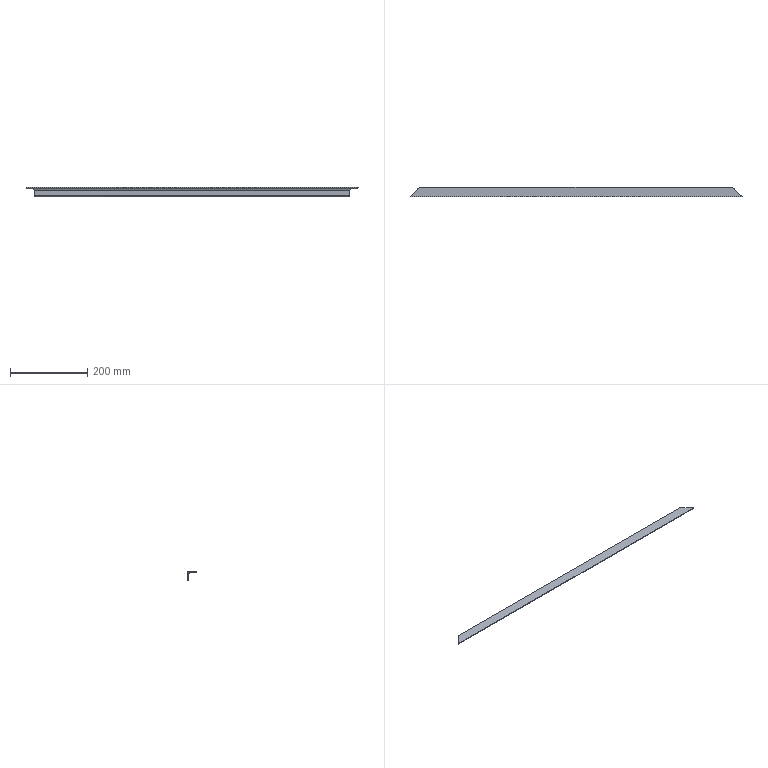Part | STEP file | Guide wheel mechanism revised.sldasm-Part-17 | 1 solid | 9 faces | box 860 x 25 x 25 mm | volume 148281 mm3 | plane 6 | cylinder 3 | commonest cylinder face diameters 8 x2 7 x1
STEP:
#1=CARTESIAN_POINT('',(-430.,795.,-505.));
#2=VERTEX_POINT('',#1);
#3=CARTESIAN_POINT('',(-405.,820.,-505.));
#4=VERTEX_POINT('',#3);
#5=CARTESIAN_POINT('',(-12.5,1212.5,-505.));
#6=DIRECTION('',(0.7071,0.7071,0.));
#7=VECTOR('',#6,1000.);
#8=LINE('',#5,#7);
#9=EDGE_CURVE('',#2,#4,#8,.T.);
#10=ORIENTED_EDGE('',*,*,#9,.F.);
#11=CARTESIAN_POINT('',(430.,795.,-505.));
#12=VERTEX_POINT('',#11);
#13=CARTESIAN_POINT('',(405.,795.,-505.));
#14=DIRECTION('',(-1.,0.,0.));
#15=VECTOR('',#14,1000.);
#16=LINE('',#13,#15);
#17=EDGE_CURVE('',#12,#2,#16,.T.);
#18=ORIENTED_EDGE('',*,*,#17,.F.);
#19=CARTESIAN_POINT('',(405.,820.,-505.));
#20=VERTEX_POINT('',#19);
#21=CARTESIAN_POINT('',(417.5,807.5,-505.));
#22=DIRECTION('',(0.7071,-0.7071,0.));
#23=VECTOR('',#22,1000.);
#24=LINE('',#21,#23);
#25=EDGE_CURVE('',#20,#12,#24,.T.);
#26=ORIENTED_EDGE('',*,*,#25,.F.);
#27=CARTESIAN_POINT('',(405.,820.,-505.));
#28=DIRECTION('',(-1.,0.,0.));
#29=VECTOR('',#28,1000.);
#30=LINE('',#27,#29);
#31=EDGE_CURVE('',#20,#4,#30,.T.);
#32=ORIENTED_EDGE('',*,*,#31,.T.);
#33=EDGE_LOOP('',(#10,#18,#26,#32));
#34=FACE_OUTER_BOUND('',#33,.T.);
#35=CARTESIAN_POINT('',(405.,795.,-505.));
#36=DIRECTION('',(0.,0.,-1.));
#37=DIRECTION('',(-1.,0.,0.));
#38=AXIS2_PLACEMENT_3D('',#35,#36,#37);
#39=PLANE('',#38);
#40=ADVANCED_FACE('',(#34),#39,.F.);
#41=CARTESIAN_POINT('',(-426.,799.,-509.));
#42=VERTEX_POINT('',#41);
#43=CARTESIAN_POINT('',(-426.,799.,-509.));
#44=CARTESIAN_POINT('',(-428.343,796.657,-509.));
#45=CARTESIAN_POINT('',(-430.,795.,-507.343));
#46=CARTESIAN_POINT('',(-430.,795.,-505.));
#47=(BOUNDED_CURVE()B_SPLINE_CURVE(3,(#43,#44,#45,#46),.UNSPECIFIED.,.F.,.F.)B_SPLINE_CURVE_WITH_KNOTS((4,4),(4.712,6.283),.UNSPECIFIED.)CURVE()GEOMETRIC_REPRESENTATION_ITEM()RATIONAL_B_SPLINE_CURVE((1.,0.8047,0.8047,1.))REPRESENTATION_ITEM(''));
#48=EDGE_CURVE('',#42,#2,#47,.T.);
#49=ORIENTED_EDGE('',*,*,#48,.F.);
#50=CARTESIAN_POINT('',(426.,799.,-509.));
#51=VERTEX_POINT('',#50);
#52=CARTESIAN_POINT('',(405.,799.,-509.));
#53=DIRECTION('',(-1.,0.,0.));
#54=VECTOR('',#53,1000.);
#55=LINE('',#52,#54);
#56=EDGE_CURVE('',#51,#42,#55,.T.);
#57=ORIENTED_EDGE('',*,*,#56,.F.);
#58=CARTESIAN_POINT('',(430.,795.,-505.));
#59=CARTESIAN_POINT('',(430.,795.,-507.343));
#60=CARTESIAN_POINT('',(428.343,796.657,-509.));
#61=CARTESIAN_POINT('',(426.,799.,-509.));
#62=(BOUNDED_CURVE()B_SPLINE_CURVE(3,(#58,#59,#60,#61),.UNSPECIFIED.,.F.,.F.)B_SPLINE_CURVE_WITH_KNOTS((4,4),(3.142,4.712),.UNSPECIFIED.)CURVE()GEOMETRIC_REPRESENTATION_ITEM()RATIONAL_B_SPLINE_CURVE((1.,0.8047,0.8047,1.))REPRESENTATION_ITEM(''));
#63=EDGE_CURVE('',#12,#51,#62,.T.);
#64=ORIENTED_EDGE('',*,*,#63,.F.);
#65=ORIENTED_EDGE('',*,*,#17,.T.);
#66=EDGE_LOOP('',(#49,#57,#64,#65));
#67=FACE_OUTER_BOUND('',#66,.T.);
#68=CARTESIAN_POINT('',(405.,799.,-505.));
#69=DIRECTION('',(-1.,0.,0.));
#70=DIRECTION('',(0.,0.,1.));
#71=AXIS2_PLACEMENT_3D('',#68,#69,#70);
#72=CYLINDRICAL_SURFACE('',#71,4.);
#73=ADVANCED_FACE('',(#67),#72,.T.);
#74=CARTESIAN_POINT('',(-412.5,812.5,-509.));
#75=VERTEX_POINT('',#74);
#76=CARTESIAN_POINT('',(-3.75,1221.25,-509.));
#77=DIRECTION('',(-0.7071,-0.7071,0.));
#78=VECTOR('',#77,1000.);
#79=LINE('',#76,#78);
#80=EDGE_CURVE('',#75,#42,#79,.T.);
#81=ORIENTED_EDGE('',*,*,#80,.F.);
#82=CARTESIAN_POINT('',(412.5,812.5,-509.));
#83=VERTEX_POINT('',#82);
#84=CARTESIAN_POINT('',(405.,812.5,-509.));
#85=DIRECTION('',(-1.,0.,0.));
#86=VECTOR('',#85,1000.);
#87=LINE('',#84,#86);
#88=EDGE_CURVE('',#83,#75,#87,.T.);
#89=ORIENTED_EDGE('',*,*,#88,.F.);
#90=CARTESIAN_POINT('',(408.75,816.25,-509.));
#91=DIRECTION('',(-0.7071,0.7071,0.));
#92=VECTOR('',#91,1000.);
#93=LINE('',#90,#92);
#94=EDGE_CURVE('',#51,#83,#93,.T.);
#95=ORIENTED_EDGE('',*,*,#94,.F.);
#96=ORIENTED_EDGE('',*,*,#56,.T.);
#97=EDGE_LOOP('',(#81,#89,#95,#96));
#98=FACE_OUTER_BOUND('',#97,.T.);
#99=CARTESIAN_POINT('',(405.,812.5,-509.));
#100=DIRECTION('',(0.,0.,1.));
#101=DIRECTION('',(1.,0.,0.));
#102=AXIS2_PLACEMENT_3D('',#99,#100,#101);
#103=PLANE('',#102);
#104=ADVANCED_FACE('',(#98),#103,.F.);
#105=CARTESIAN_POINT('',(-409.,816.,-512.5));
#106=VERTEX_POINT('',#105);
#107=CARTESIAN_POINT('',(-409.,816.,-512.5));
#108=CARTESIAN_POINT('',(-409.,816.,-510.45));
#109=CARTESIAN_POINT('',(-410.45,814.55,-509.));
#110=CARTESIAN_POINT('',(-412.5,812.5,-509.));
#111=(BOUNDED_CURVE()B_SPLINE_CURVE(3,(#107,#108,#109,#110),.UNSPECIFIED.,.F.,.F.)B_SPLINE_CURVE_WITH_KNOTS((4,4),(3.142,4.712),.UNSPECIFIED.)CURVE()GEOMETRIC_REPRESENTATION_ITEM()RATIONAL_B_SPLINE_CURVE((1.,0.8047,0.8047,1.))REPRESENTATION_ITEM(''));
#112=EDGE_CURVE('',#106,#75,#111,.T.);
#113=ORIENTED_EDGE('',*,*,#112,.F.);
#114=CARTESIAN_POINT('',(409.,816.,-512.5));
#115=VERTEX_POINT('',#114);
#116=CARTESIAN_POINT('',(405.,816.,-512.5));
#117=DIRECTION('',(-1.,0.,0.));
#118=VECTOR('',#117,1000.);
#119=LINE('',#116,#118);
#120=EDGE_CURVE('',#115,#106,#119,.T.);
#121=ORIENTED_EDGE('',*,*,#120,.F.);
#122=CARTESIAN_POINT('',(412.5,812.5,-509.));
#123=CARTESIAN_POINT('',(410.45,814.55,-509.));
#124=CARTESIAN_POINT('',(409.,816.,-510.45));
#125=CARTESIAN_POINT('',(409.,816.,-512.5));
#126=(BOUNDED_CURVE()B_SPLINE_CURVE(3,(#122,#123,#124,#125),.UNSPECIFIED.,.F.,.F.)B_SPLINE_CURVE_WITH_KNOTS((4,4),(4.712,6.283),.UNSPECIFIED.)CURVE()GEOMETRIC_REPRESENTATION_ITEM()RATIONAL_B_SPLINE_CURVE((1.,0.8047,0.8047,1.))REPRESENTATION_ITEM(''));
#127=EDGE_CURVE('',#83,#115,#126,.T.);
#128=ORIENTED_EDGE('',*,*,#127,.F.);
#129=ORIENTED_EDGE('',*,*,#88,.T.);
#130=EDGE_LOOP('',(#113,#121,#128,#129));
#131=FACE_OUTER_BOUND('',#130,.T.);
#132=CARTESIAN_POINT('',(405.,812.5,-512.5));
#133=DIRECTION('',(-1.,0.,0.));
#134=DIRECTION('',(0.,0.,1.));
#135=AXIS2_PLACEMENT_3D('',#132,#133,#134);
#136=CYLINDRICAL_SURFACE('',#135,3.5);
#137=ADVANCED_FACE('',(#131),#136,.F.);
#138=CARTESIAN_POINT('',(-409.,816.,-526.));
#139=VERTEX_POINT('',#138);
#140=CARTESIAN_POINT('',(-409.,816.,-526.));
#141=DIRECTION('',(0.,0.,1.));
#142=VECTOR('',#141,1000.);
#143=LINE('',#140,#142);
#144=EDGE_CURVE('',#139,#106,#143,.T.);
#145=ORIENTED_EDGE('',*,*,#144,.F.);
#146=CARTESIAN_POINT('',(409.,816.,-526.));
#147=VERTEX_POINT('',#146);
#148=CARTESIAN_POINT('',(405.,816.,-526.));
#149=DIRECTION('',(-1.,0.,0.));
#150=VECTOR('',#149,1000.);
#151=LINE('',#148,#150);
#152=EDGE_CURVE('',#147,#139,#151,.T.);
#153=ORIENTED_EDGE('',*,*,#152,.F.);
#154=CARTESIAN_POINT('',(409.,816.,-526.));
#155=DIRECTION('',(0.,0.,-1.));
#156=VECTOR('',#155,1000.);
#157=LINE('',#154,#156);
#158=EDGE_CURVE('',#115,#147,#157,.T.);
#159=ORIENTED_EDGE('',*,*,#158,.F.);
#160=ORIENTED_EDGE('',*,*,#120,.T.);
#161=EDGE_LOOP('',(#145,#153,#159,#160));
#162=FACE_OUTER_BOUND('',#161,.T.);
#163=CARTESIAN_POINT('',(405.,816.,-526.));
#164=DIRECTION('',(0.,1.,0.));
#165=DIRECTION('',(0.,0.,1.));
#166=AXIS2_PLACEMENT_3D('',#163,#164,#165);
#167=PLANE('',#166);
#168=ADVANCED_FACE('',(#162),#167,.F.);
#169=CARTESIAN_POINT('',(-405.,820.,-530.));
#170=VERTEX_POINT('',#169);
#171=CARTESIAN_POINT('',(-405.,820.,-530.));
#172=CARTESIAN_POINT('',(-407.343,817.657,-530.));
#173=CARTESIAN_POINT('',(-409.,816.,-528.343));
#174=CARTESIAN_POINT('',(-409.,816.,-526.));
#175=(BOUNDED_CURVE()B_SPLINE_CURVE(3,(#171,#172,#173,#174),.UNSPECIFIED.,.F.,.F.)B_SPLINE_CURVE_WITH_KNOTS((4,4),(4.712,6.283),.UNSPECIFIED.)CURVE()GEOMETRIC_REPRESENTATION_ITEM()RATIONAL_B_SPLINE_CURVE((1.,0.8047,0.8047,1.))REPRESENTATION_ITEM(''));
#176=EDGE_CURVE('',#170,#139,#175,.T.);
#177=ORIENTED_EDGE('',*,*,#176,.F.);
#178=CARTESIAN_POINT('',(405.,820.,-530.));
#179=VERTEX_POINT('',#178);
#180=CARTESIAN_POINT('',(405.,820.,-530.));
#181=DIRECTION('',(-1.,0.,0.));
#182=VECTOR('',#181,1000.);
#183=LINE('',#180,#182);
#184=EDGE_CURVE('',#179,#170,#183,.T.);
#185=ORIENTED_EDGE('',*,*,#184,.F.);
#186=CARTESIAN_POINT('',(409.,816.,-526.));
#187=CARTESIAN_POINT('',(409.,816.,-528.343));
#188=CARTESIAN_POINT('',(407.343,817.657,-530.));
#189=CARTESIAN_POINT('',(405.,820.,-530.));
#190=(BOUNDED_CURVE()B_SPLINE_CURVE(3,(#186,#187,#188,#189),.UNSPECIFIED.,.F.,.T.)B_SPLINE_CURVE_WITH_KNOTS((4,4),(3.142,4.712),.UNSPECIFIED.)CURVE()GEOMETRIC_REPRESENTATION_ITEM()RATIONAL_B_SPLINE_CURVE((1.,0.8047,0.8047,1.))REPRESENTATION_ITEM(''));
#191=EDGE_CURVE('',#147,#179,#190,.T.);
#192=ORIENTED_EDGE('',*,*,#191,.F.);
#193=ORIENTED_EDGE('',*,*,#152,.T.);
#194=EDGE_LOOP('',(#177,#185,#192,#193));
#195=FACE_OUTER_BOUND('',#194,.T.);
#196=CARTESIAN_POINT('',(405.,820.,-526.));
#197=DIRECTION('',(-1.,0.,0.));
#198=DIRECTION('',(0.,0.,1.));
#199=AXIS2_PLACEMENT_3D('',#196,#197,#198);
#200=CYLINDRICAL_SURFACE('',#199,4.);
#201=ADVANCED_FACE('',(#195),#200,.T.);
#202=CARTESIAN_POINT('',(-405.,820.,-505.));
#203=DIRECTION('',(0.,0.,-1.));
#204=VECTOR('',#203,1000.);
#205=LINE('',#202,#204);
#206=EDGE_CURVE('',#4,#170,#205,.T.);
#207=ORIENTED_EDGE('',*,*,#206,.F.);
#208=ORIENTED_EDGE('',*,*,#31,.F.);
#209=CARTESIAN_POINT('',(405.,820.,-505.));
#210=DIRECTION('',(0.,0.,1.));
#211=VECTOR('',#210,1000.);
#212=LINE('',#209,#211);
#213=EDGE_CURVE('',#179,#20,#212,.T.);
#214=ORIENTED_EDGE('',*,*,#213,.F.);
#215=ORIENTED_EDGE('',*,*,#184,.T.);
#216=EDGE_LOOP('',(#207,#208,#214,#215));
#217=FACE_OUTER_BOUND('',#216,.T.);
#218=CARTESIAN_POINT('',(405.,820.,-505.));
#219=DIRECTION('',(0.,-1.,0.));
#220=DIRECTION('',(0.,0.,-1.));
#221=AXIS2_PLACEMENT_3D('',#218,#219,#220);
#222=PLANE('',#221);
#223=ADVANCED_FACE('',(#217),#222,.F.);
#224=ORIENTED_EDGE('',*,*,#213,.T.);
#225=ORIENTED_EDGE('',*,*,#25,.T.);
#226=ORIENTED_EDGE('',*,*,#63,.T.);
#227=ORIENTED_EDGE('',*,*,#94,.T.);
#228=ORIENTED_EDGE('',*,*,#127,.T.);
#229=ORIENTED_EDGE('',*,*,#158,.T.);
#230=ORIENTED_EDGE('',*,*,#191,.T.);
#231=EDGE_LOOP('',(#224,#225,#226,#227,#228,#229,#230));
#232=FACE_OUTER_BOUND('',#231,.T.);
#233=CARTESIAN_POINT('',(405.,820.,-505.));
#234=DIRECTION('',(0.7071,0.7071,0.));
#235=DIRECTION('',(-0.7071,0.7071,0.));
#236=AXIS2_PLACEMENT_3D('',#233,#234,#235);
#237=PLANE('',#236);
#238=ADVANCED_FACE('',(#232),#237,.T.);
#239=ORIENTED_EDGE('',*,*,#48,.T.);
#240=ORIENTED_EDGE('',*,*,#9,.T.);
#241=ORIENTED_EDGE('',*,*,#206,.T.);
#242=ORIENTED_EDGE('',*,*,#176,.T.);
#243=ORIENTED_EDGE('',*,*,#144,.T.);
#244=ORIENTED_EDGE('',*,*,#112,.T.);
#245=ORIENTED_EDGE('',*,*,#80,.T.);
#246=EDGE_LOOP('',(#239,#240,#241,#242,#243,#244,#245));
#247=FACE_OUTER_BOUND('',#246,.T.);
#248=CARTESIAN_POINT('',(-405.,820.,-505.));
#249=DIRECTION('',(-0.7071,0.7071,0.));
#250=DIRECTION('',(-0.7071,-0.7071,0.));
#251=AXIS2_PLACEMENT_3D('',#248,#249,#250);
#252=PLANE('',#251);
#253=ADVANCED_FACE('',(#247),#252,.T.);
#254=CLOSED_SHELL('',(#40,#73,#104,#137,#168,#201,#223,#238,#253));
#255=MANIFOLD_SOLID_BREP('',#254);
#256=CARTESIAN_POINT('',(0.,0.,0.));
#257=DIRECTION('',(0.,0.,1.));
#258=DIRECTION('',(1.,0.,0.));
#259=AXIS2_PLACEMENT_3D('',#256,#257,#258);
#260=(LENGTH_UNIT()NAMED_UNIT(*)SI_UNIT(.MILLI.,.METRE.));
#261=UNCERTAINTY_MEASURE_WITH_UNIT(LENGTH_MEASURE(0.00001),#260,'','');
#262=(NAMED_UNIT(*)PLANE_ANGLE_UNIT()SI_UNIT($,.RADIAN.));
#263=(NAMED_UNIT(*)SI_UNIT($,.STERADIAN.)SOLID_ANGLE_UNIT());
#264=(GEOMETRIC_REPRESENTATION_CONTEXT(3)GLOBAL_UNCERTAINTY_ASSIGNED_CONTEXT((#261))GLOBAL_UNIT_ASSIGNED_CONTEXT((#260,#262,#263))REPRESENTATION_CONTEXT('',''));
#265=ADVANCED_BREP_SHAPE_REPRESENTATION('',(#255,#259),#264);